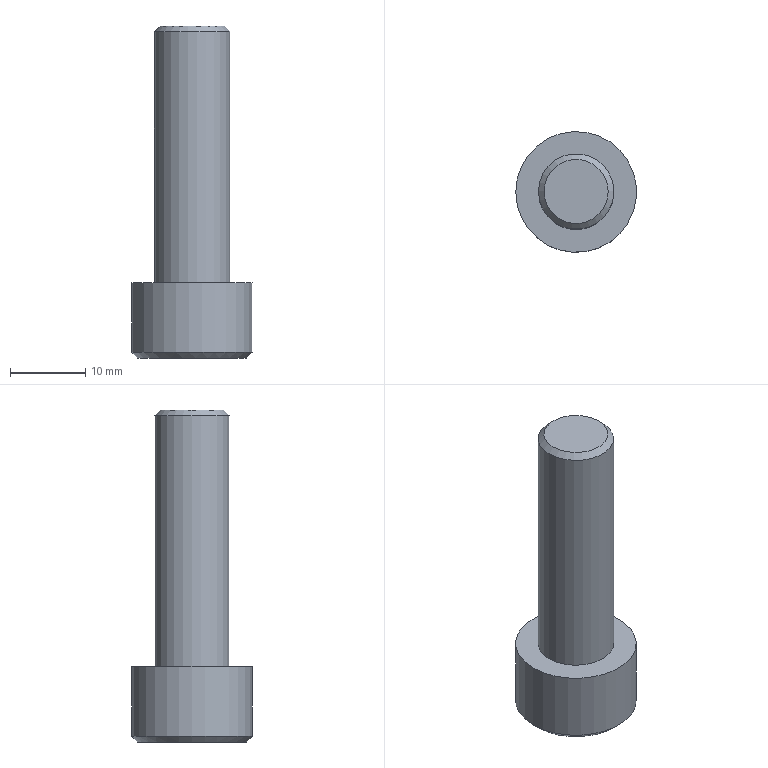Part | STEP file | M10.00-35.00 | 1 solid | 14 faces | box 16 x 16 x 44 mm | volume 4346 mm3 | plane 10 | cylinder 2 | cone 2 | commonest cylinder face diameters 10 x1 16 x1